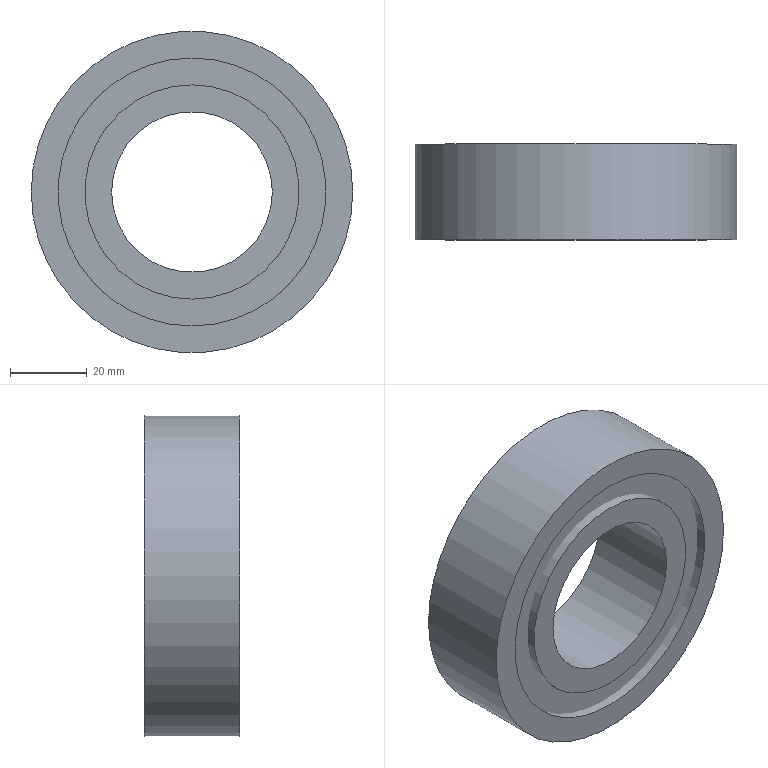Part | NX | features DATUM_CSYS 4, EXTRUDE 3, SKETCH 3 | 3 solids | 12 faces | box 84 x 25 x 84 mm | volume 100939 mm3 | plane 6 | cylinder 6 | commonest cylinder face diameters 42 x1 55 x1 56 x1 70 x1 71 x1 84 x1
STEP:
#1=CARTESIAN_POINT('',(0.,-25.,35.));
#2=VERTEX_POINT('',#1);
#3=CARTESIAN_POINT('',(0.,-25.,0.));
#4=DIRECTION('',(0.,1.,0.));
#5=DIRECTION('',(0.,0.,1.));
#6=AXIS2_PLACEMENT_3D('',#3,#4,#5);
#7=CIRCLE('',#6,35.);
#8=EDGE_CURVE('',#2,#2,#7,.F.);
#9=ORIENTED_EDGE('',*,*,#8,.F.);
#10=EDGE_LOOP('',(#9));
#11=FACE_BOUND('',#10,.T.);
#12=CARTESIAN_POINT('',(42.,-25.,0.));
#13=VERTEX_POINT('',#12);
#14=CARTESIAN_POINT('',(0.,-25.,0.));
#15=DIRECTION('',(0.,-1.,0.));
#16=DIRECTION('',(1.,0.,0.));
#17=AXIS2_PLACEMENT_3D('',#14,#15,#16);
#18=CIRCLE('',#17,42.);
#19=EDGE_CURVE('',#13,#13,#18,.T.);
#20=ORIENTED_EDGE('',*,*,#19,.T.);
#21=EDGE_LOOP('',(#20));
#22=FACE_BOUND('',#21,.T.);
#23=CARTESIAN_POINT('',(0.,-25.,0.));
#24=DIRECTION('',(0.,1.,0.));
#25=DIRECTION('',(0.,0.,1.));
#26=AXIS2_PLACEMENT_3D('',#23,#24,#25);
#27=PLANE('',#26);
#28=ADVANCED_FACE('',(#11,#22),#27,.F.);
#29=CARTESIAN_POINT('',(0.,0.,35.));
#30=VERTEX_POINT('',#29);
#31=CARTESIAN_POINT('',(0.,0.,0.));
#32=DIRECTION('',(0.,1.,0.));
#33=DIRECTION('',(0.,0.,1.));
#34=AXIS2_PLACEMENT_3D('',#31,#32,#33);
#35=CIRCLE('',#34,35.);
#36=EDGE_CURVE('',#30,#30,#35,.F.);
#37=ORIENTED_EDGE('',*,*,#36,.T.);
#38=EDGE_LOOP('',(#37));
#39=FACE_BOUND('',#38,.T.);
#40=CARTESIAN_POINT('',(42.,0.,0.));
#41=VERTEX_POINT('',#40);
#42=CARTESIAN_POINT('',(0.,0.,0.));
#43=DIRECTION('',(0.,-1.,0.));
#44=DIRECTION('',(1.,0.,0.));
#45=AXIS2_PLACEMENT_3D('',#42,#43,#44);
#46=CIRCLE('',#45,42.);
#47=EDGE_CURVE('',#41,#41,#46,.T.);
#48=ORIENTED_EDGE('',*,*,#47,.F.);
#49=EDGE_LOOP('',(#48));
#50=FACE_BOUND('',#49,.T.);
#51=CARTESIAN_POINT('',(0.,0.,0.));
#52=DIRECTION('',(0.,1.,0.));
#53=DIRECTION('',(0.,0.,1.));
#54=AXIS2_PLACEMENT_3D('',#51,#52,#53);
#55=PLANE('',#54);
#56=ADVANCED_FACE('',(#39,#50),#55,.T.);
#57=ORIENTED_EDGE('',*,*,#8,.T.);
#58=EDGE_LOOP('',(#57));
#59=FACE_BOUND('',#58,.T.);
#60=ORIENTED_EDGE('',*,*,#36,.F.);
#61=EDGE_LOOP('',(#60));
#62=FACE_BOUND('',#61,.T.);
#63=CARTESIAN_POINT('',(0.,-25.,0.));
#64=DIRECTION('',(0.,1.,0.));
#65=DIRECTION('',(0.,0.,1.));
#66=AXIS2_PLACEMENT_3D('',#63,#64,#65);
#67=CYLINDRICAL_SURFACE('',#66,35.);
#68=ADVANCED_FACE('',(#59,#62),#67,.F.);
#69=ORIENTED_EDGE('',*,*,#19,.F.);
#70=EDGE_LOOP('',(#69));
#71=FACE_BOUND('',#70,.T.);
#72=ORIENTED_EDGE('',*,*,#47,.T.);
#73=EDGE_LOOP('',(#72));
#74=FACE_BOUND('',#73,.T.);
#75=CARTESIAN_POINT('',(0.,-25.,0.));
#76=DIRECTION('',(0.,1.,0.));
#77=DIRECTION('',(0.,0.,1.));
#78=AXIS2_PLACEMENT_3D('',#75,#76,#77);
#79=CYLINDRICAL_SURFACE('',#78,42.);
#80=ADVANCED_FACE('',(#71,#74),#79,.T.);
#81=CLOSED_SHELL('',(#28,#56,#68,#80));
#82=MANIFOLD_SOLID_BREP('',#81);
#83=CARTESIAN_POINT('',(0.,-25.,28.));
#84=VERTEX_POINT('',#83);
#85=CARTESIAN_POINT('',(0.,-25.,0.));
#86=DIRECTION('',(0.,1.,0.));
#87=DIRECTION('',(0.,0.,1.));
#88=AXIS2_PLACEMENT_3D('',#85,#86,#87);
#89=CIRCLE('',#88,28.);
#90=EDGE_CURVE('',#84,#84,#89,.T.);
#91=ORIENTED_EDGE('',*,*,#90,.F.);
#92=EDGE_LOOP('',(#91));
#93=FACE_BOUND('',#92,.T.);
#94=CARTESIAN_POINT('',(21.,-25.,0.));
#95=VERTEX_POINT('',#94);
#96=CARTESIAN_POINT('',(0.,-25.,0.));
#97=DIRECTION('',(0.,-1.,0.));
#98=DIRECTION('',(1.,0.,0.));
#99=AXIS2_PLACEMENT_3D('',#96,#97,#98);
#100=CIRCLE('',#99,21.);
#101=EDGE_CURVE('',#95,#95,#100,.F.);
#102=ORIENTED_EDGE('',*,*,#101,.T.);
#103=EDGE_LOOP('',(#102));
#104=FACE_BOUND('',#103,.T.);
#105=CARTESIAN_POINT('',(0.,-25.,0.));
#106=DIRECTION('',(0.,1.,0.));
#107=DIRECTION('',(0.,0.,1.));
#108=AXIS2_PLACEMENT_3D('',#105,#106,#107);
#109=PLANE('',#108);
#110=ADVANCED_FACE('',(#93,#104),#109,.F.);
#111=CARTESIAN_POINT('',(0.,0.,28.));
#112=VERTEX_POINT('',#111);
#113=CARTESIAN_POINT('',(0.,0.,0.));
#114=DIRECTION('',(0.,1.,0.));
#115=DIRECTION('',(0.,0.,1.));
#116=AXIS2_PLACEMENT_3D('',#113,#114,#115);
#117=CIRCLE('',#116,28.);
#118=EDGE_CURVE('',#112,#112,#117,.T.);
#119=ORIENTED_EDGE('',*,*,#118,.T.);
#120=EDGE_LOOP('',(#119));
#121=FACE_BOUND('',#120,.T.);
#122=CARTESIAN_POINT('',(21.,0.,0.));
#123=VERTEX_POINT('',#122);
#124=CARTESIAN_POINT('',(0.,0.,0.));
#125=DIRECTION('',(0.,-1.,0.));
#126=DIRECTION('',(1.,0.,0.));
#127=AXIS2_PLACEMENT_3D('',#124,#125,#126);
#128=CIRCLE('',#127,21.);
#129=EDGE_CURVE('',#123,#123,#128,.F.);
#130=ORIENTED_EDGE('',*,*,#129,.F.);
#131=EDGE_LOOP('',(#130));
#132=FACE_BOUND('',#131,.T.);
#133=CARTESIAN_POINT('',(0.,0.,0.));
#134=DIRECTION('',(0.,1.,0.));
#135=DIRECTION('',(0.,0.,1.));
#136=AXIS2_PLACEMENT_3D('',#133,#134,#135);
#137=PLANE('',#136);
#138=ADVANCED_FACE('',(#121,#132),#137,.T.);
#139=ORIENTED_EDGE('',*,*,#90,.T.);
#140=EDGE_LOOP('',(#139));
#141=FACE_BOUND('',#140,.T.);
#142=ORIENTED_EDGE('',*,*,#118,.F.);
#143=EDGE_LOOP('',(#142));
#144=FACE_BOUND('',#143,.T.);
#145=CARTESIAN_POINT('',(0.,-25.,0.));
#146=DIRECTION('',(0.,1.,0.));
#147=DIRECTION('',(0.,0.,1.));
#148=AXIS2_PLACEMENT_3D('',#145,#146,#147);
#149=CYLINDRICAL_SURFACE('',#148,28.);
#150=ADVANCED_FACE('',(#141,#144),#149,.T.);
#151=ORIENTED_EDGE('',*,*,#101,.F.);
#152=EDGE_LOOP('',(#151));
#153=FACE_BOUND('',#152,.T.);
#154=ORIENTED_EDGE('',*,*,#129,.T.);
#155=EDGE_LOOP('',(#154));
#156=FACE_BOUND('',#155,.T.);
#157=CARTESIAN_POINT('',(0.,-25.,0.));
#158=DIRECTION('',(0.,1.,0.));
#159=DIRECTION('',(0.,0.,1.));
#160=AXIS2_PLACEMENT_3D('',#157,#158,#159);
#161=CYLINDRICAL_SURFACE('',#160,21.);
#162=ADVANCED_FACE('',(#153,#156),#161,.F.);
#163=CLOSED_SHELL('',(#110,#138,#150,#162));
#164=MANIFOLD_SOLID_BREP('',#163);
#165=CARTESIAN_POINT('',(0.,-2.5,-27.5));
#166=VERTEX_POINT('',#165);
#167=CARTESIAN_POINT('',(0.,-2.5,0.));
#168=DIRECTION('',(0.,-1.,0.));
#169=DIRECTION('',(0.,0.,-1.));
#170=AXIS2_PLACEMENT_3D('',#167,#168,#169);
#171=CIRCLE('',#170,27.5);
#172=EDGE_CURVE('',#166,#166,#171,.T.);
#173=ORIENTED_EDGE('',*,*,#172,.T.);
#174=EDGE_LOOP('',(#173));
#175=FACE_BOUND('',#174,.T.);
#176=CARTESIAN_POINT('',(0.,-2.5,-35.5));
#177=VERTEX_POINT('',#176);
#178=CARTESIAN_POINT('',(0.,-2.5,0.));
#179=DIRECTION('',(0.,-1.,0.));
#180=DIRECTION('',(0.,0.,-1.));
#181=AXIS2_PLACEMENT_3D('',#178,#179,#180);
#182=CIRCLE('',#181,35.5);
#183=EDGE_CURVE('',#177,#177,#182,.T.);
#184=ORIENTED_EDGE('',*,*,#183,.F.);
#185=EDGE_LOOP('',(#184));
#186=FACE_BOUND('',#185,.T.);
#187=CARTESIAN_POINT('',(0.,-2.5,0.));
#188=DIRECTION('',(0.,-1.,0.));
#189=DIRECTION('',(0.,0.,-1.));
#190=AXIS2_PLACEMENT_3D('',#187,#188,#189);
#191=PLANE('',#190);
#192=ADVANCED_FACE('',(#175,#186),#191,.F.);
#193=CARTESIAN_POINT('',(0.,-22.5,-27.5));
#194=VERTEX_POINT('',#193);
#195=CARTESIAN_POINT('',(0.,-22.5,0.));
#196=DIRECTION('',(0.,-1.,0.));
#197=DIRECTION('',(0.,0.,-1.));
#198=AXIS2_PLACEMENT_3D('',#195,#196,#197);
#199=CIRCLE('',#198,27.5);
#200=EDGE_CURVE('',#194,#194,#199,.T.);
#201=ORIENTED_EDGE('',*,*,#200,.F.);
#202=EDGE_LOOP('',(#201));
#203=FACE_BOUND('',#202,.T.);
#204=CARTESIAN_POINT('',(0.,-22.5,-35.5));
#205=VERTEX_POINT('',#204);
#206=CARTESIAN_POINT('',(0.,-22.5,0.));
#207=DIRECTION('',(0.,-1.,0.));
#208=DIRECTION('',(0.,0.,-1.));
#209=AXIS2_PLACEMENT_3D('',#206,#207,#208);
#210=CIRCLE('',#209,35.5);
#211=EDGE_CURVE('',#205,#205,#210,.T.);
#212=ORIENTED_EDGE('',*,*,#211,.T.);
#213=EDGE_LOOP('',(#212));
#214=FACE_BOUND('',#213,.T.);
#215=CARTESIAN_POINT('',(0.,-22.5,0.));
#216=DIRECTION('',(0.,-1.,0.));
#217=DIRECTION('',(0.,0.,-1.));
#218=AXIS2_PLACEMENT_3D('',#215,#216,#217);
#219=PLANE('',#218);
#220=ADVANCED_FACE('',(#203,#214),#219,.T.);
#221=ORIENTED_EDGE('',*,*,#172,.F.);
#222=EDGE_LOOP('',(#221));
#223=FACE_BOUND('',#222,.T.);
#224=ORIENTED_EDGE('',*,*,#200,.T.);
#225=EDGE_LOOP('',(#224));
#226=FACE_BOUND('',#225,.T.);
#227=CARTESIAN_POINT('',(0.,-2.5,0.));
#228=DIRECTION('',(0.,-1.,0.));
#229=DIRECTION('',(0.,0.,-1.));
#230=AXIS2_PLACEMENT_3D('',#227,#228,#229);
#231=CYLINDRICAL_SURFACE('',#230,27.5);
#232=ADVANCED_FACE('',(#223,#226),#231,.F.);
#233=ORIENTED_EDGE('',*,*,#183,.T.);
#234=EDGE_LOOP('',(#233));
#235=FACE_BOUND('',#234,.T.);
#236=ORIENTED_EDGE('',*,*,#211,.F.);
#237=EDGE_LOOP('',(#236));
#238=FACE_BOUND('',#237,.T.);
#239=CARTESIAN_POINT('',(0.,-2.5,0.));
#240=DIRECTION('',(0.,-1.,0.));
#241=DIRECTION('',(0.,0.,-1.));
#242=AXIS2_PLACEMENT_3D('',#239,#240,#241);
#243=CYLINDRICAL_SURFACE('',#242,35.5);
#244=ADVANCED_FACE('',(#235,#238),#243,.T.);
#245=CLOSED_SHELL('',(#192,#220,#232,#244));
#246=MANIFOLD_SOLID_BREP('',#245);
#247=(LENGTH_UNIT()NAMED_UNIT(*)SI_UNIT(.MILLI.,.METRE.));
#248=UNCERTAINTY_MEASURE_WITH_UNIT(LENGTH_MEASURE(0.00001),#247,'','');
#249=(NAMED_UNIT(*)PLANE_ANGLE_UNIT()SI_UNIT($,.RADIAN.));
#250=(NAMED_UNIT(*)SI_UNIT($,.STERADIAN.)SOLID_ANGLE_UNIT());
#251=(GEOMETRIC_REPRESENTATION_CONTEXT(3)GLOBAL_UNCERTAINTY_ASSIGNED_CONTEXT((#248))GLOBAL_UNIT_ASSIGNED_CONTEXT((#247,#249,#250))REPRESENTATION_CONTEXT('',''));
#252=ADVANCED_BREP_SHAPE_REPRESENTATION('',(#82,#164,#246),#251);